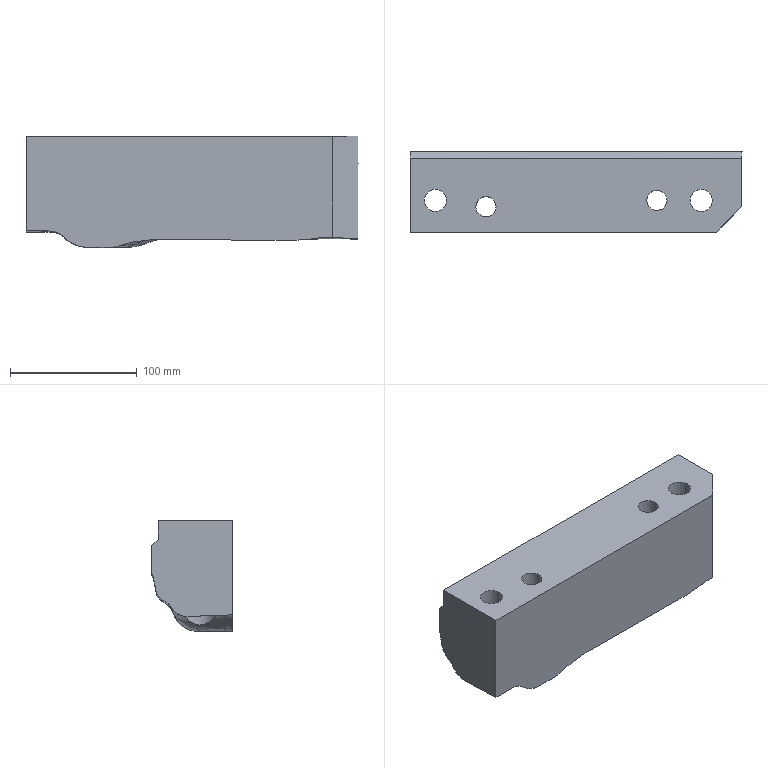Part | NX | features solid 2 | 1 solid | 55 faces | volume 1111766 mm3 | spline 42 | plane 7 | cylinder 6 | commonest cylinder face diameters 16 x2 17.5 x2 25.5 x2